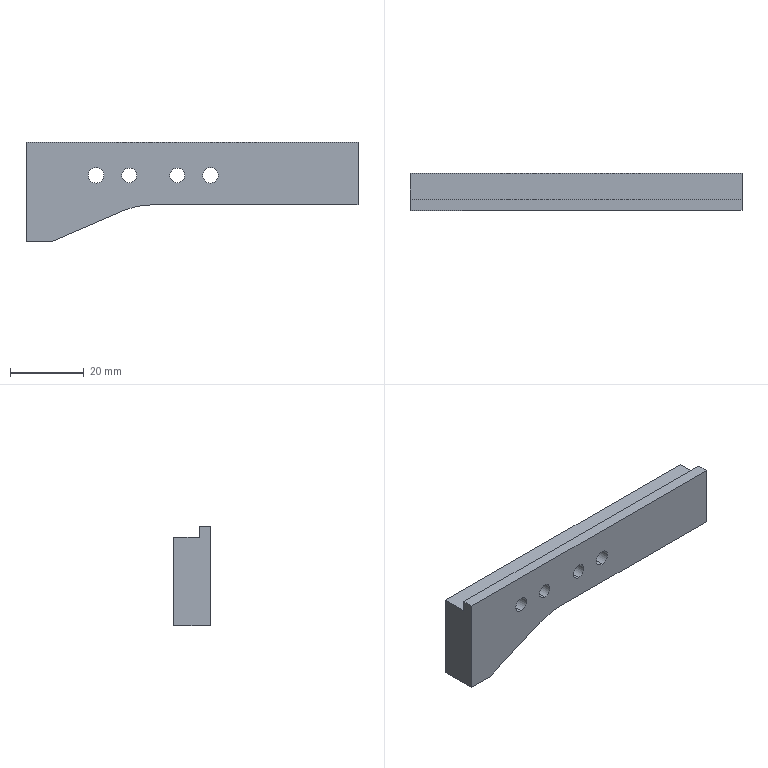Part | STEP file | PN_0060 | 1 solid | 19 faces | box 90 x 10 x 27 mm | volume 14739 mm3 | plane 10 | cylinder 9 | commonest cylinder face diameters 4 x4 4.2 x4 40 x1
STEP:
#1=CARTESIAN_POINT('',(0.,0.,0.));
#2=DIRECTION('',(0.,0.,1.));
#3=DIRECTION('',(1.,0.,0.));
#4=AXIS2_PLACEMENT_3D('',#1,#2,#3);
#5=CARTESIAN_POINT('',(-32.,0.,1.5));
#6=VERTEX_POINT('',#5);
#7=CARTESIAN_POINT('',(-32.,10.,1.5));
#8=VERTEX_POINT('',#7);
#9=CARTESIAN_POINT('',(-32.,10.,1.5));
#10=DIRECTION('',(0.,1.,0.));
#11=VECTOR('',#10,1.);
#12=LINE('',#9,#11);
#13=CARTESIAN_POINT('',(-32.,10.,-0.5));
#14=DIRECTION('',(0.,1.,0.));
#15=DIRECTION('',(0.,0.,1.));
#16=AXIS2_PLACEMENT_3D('',#13,#14,#15);
#17=CYLINDRICAL_SURFACE('',#16,2.);
#18=CARTESIAN_POINT('',(6.283,0.));
#19=DIRECTION('',(0.,1.));
#20=VECTOR('',#19,1.);
#21=LINE('',#18,#20);
#22=(GEOMETRIC_REPRESENTATION_CONTEXT(2)PARAMETRIC_REPRESENTATION_CONTEXT()REPRESENTATION_CONTEXT('',''));
#23=DEFINITIONAL_REPRESENTATION('',(#21),#22);
#24=PCURVE('',#17,#23);
#25=CARTESIAN_POINT('',(-32.,10.,-0.5));
#26=DIRECTION('',(0.,1.,0.));
#27=DIRECTION('',(0.,0.,1.));
#28=AXIS2_PLACEMENT_3D('',#25,#26,#27);
#29=CYLINDRICAL_SURFACE('',#28,2.);
#30=CARTESIAN_POINT('',(0.,0.));
#31=DIRECTION('',(0.,1.));
#32=VECTOR('',#31,1.);
#33=LINE('',#30,#32);
#34=(GEOMETRIC_REPRESENTATION_CONTEXT(2)PARAMETRIC_REPRESENTATION_CONTEXT()REPRESENTATION_CONTEXT('',''));
#35=DEFINITIONAL_REPRESENTATION('',(#33),#34);
#36=PCURVE('',#29,#35);
#37=SURFACE_CURVE('',#12,(#24,#36),.PCURVE_S1.);
#38=EDGE_CURVE('',#6,#8,#37,.T.);
#39=ORIENTED_EDGE('',*,*,#38,.T.);
#40=CARTESIAN_POINT('',(-32.,10.,-2.5));
#41=VERTEX_POINT('',#40);
#42=CARTESIAN_POINT('',(-32.,10.,-0.5));
#43=DIRECTION('',(0.,1.,0.));
#44=DIRECTION('',(0.,0.,1.));
#45=AXIS2_PLACEMENT_3D('',#42,#43,#44);
#46=CIRCLE('',#45,2.);
#47=CARTESIAN_POINT('',(0.,0.));
#48=DIRECTION('',(1.,0.));
#49=VECTOR('',#48,1.);
#50=LINE('',#47,#49);
#51=(GEOMETRIC_REPRESENTATION_CONTEXT(2)PARAMETRIC_REPRESENTATION_CONTEXT()REPRESENTATION_CONTEXT('',''));
#52=DEFINITIONAL_REPRESENTATION('',(#50),#51);
#53=PCURVE('',#17,#52);
#54=CARTESIAN_POINT('',(0.,10.,0.));
#55=DIRECTION('',(0.,1.,0.));
#56=DIRECTION('',(0.,0.,1.));
#57=AXIS2_PLACEMENT_3D('',#54,#55,#56);
#58=PLANE('',#57);
#59=CARTESIAN_POINT('',(-0.5,-32.));
#60=DIRECTION('',(1.,0.));
#61=AXIS2_PLACEMENT_2D('',#59,#60);
#62=CIRCLE('',#61,2.);
#63=(GEOMETRIC_REPRESENTATION_CONTEXT(2)PARAMETRIC_REPRESENTATION_CONTEXT()REPRESENTATION_CONTEXT('',''));
#64=DEFINITIONAL_REPRESENTATION('',(#62),#63);
#65=PCURVE('',#58,#64);
#66=SURFACE_CURVE('',#46,(#53,#65),.PCURVE_S1.);
#67=EDGE_CURVE('',#41,#8,#66,.T.);
#68=ORIENTED_EDGE('',*,*,#67,.F.);
#69=CARTESIAN_POINT('',(-32.,0.,-2.5));
#70=VERTEX_POINT('',#69);
#71=CARTESIAN_POINT('',(-32.,10.,-2.5));
#72=DIRECTION('',(0.,1.,0.));
#73=VECTOR('',#72,1.);
#74=LINE('',#71,#73);
#75=CARTESIAN_POINT('',(3.142,0.));
#76=DIRECTION('',(0.,1.));
#77=VECTOR('',#76,1.);
#78=LINE('',#75,#77);
#79=(GEOMETRIC_REPRESENTATION_CONTEXT(2)PARAMETRIC_REPRESENTATION_CONTEXT()REPRESENTATION_CONTEXT('',''));
#80=DEFINITIONAL_REPRESENTATION('',(#78),#79);
#81=PCURVE('',#17,#80);
#82=CARTESIAN_POINT('',(3.142,0.));
#83=DIRECTION('',(0.,1.));
#84=VECTOR('',#83,1.);
#85=LINE('',#82,#84);
#86=(GEOMETRIC_REPRESENTATION_CONTEXT(2)PARAMETRIC_REPRESENTATION_CONTEXT()REPRESENTATION_CONTEXT('',''));
#87=DEFINITIONAL_REPRESENTATION('',(#85),#86);
#88=PCURVE('',#29,#87);
#89=SURFACE_CURVE('',#74,(#81,#88),.PCURVE_S1.);
#90=EDGE_CURVE('',#70,#41,#89,.T.);
#91=ORIENTED_EDGE('',*,*,#90,.F.);
#92=CARTESIAN_POINT('',(-32.,0.,-0.5));
#93=DIRECTION('',(0.,1.,0.));
#94=DIRECTION('',(0.,0.,1.));
#95=AXIS2_PLACEMENT_3D('',#92,#93,#94);
#96=CIRCLE('',#95,2.);
#97=CARTESIAN_POINT('',(0.,-10.));
#98=DIRECTION('',(1.,0.));
#99=VECTOR('',#98,1.);
#100=LINE('',#97,#99);
#101=(GEOMETRIC_REPRESENTATION_CONTEXT(2)PARAMETRIC_REPRESENTATION_CONTEXT()REPRESENTATION_CONTEXT('',''));
#102=DEFINITIONAL_REPRESENTATION('',(#100),#101);
#103=PCURVE('',#17,#102);
#104=CARTESIAN_POINT('',(0.,0.,0.));
#105=DIRECTION('',(0.,1.,0.));
#106=DIRECTION('',(0.,0.,1.));
#107=AXIS2_PLACEMENT_3D('',#104,#105,#106);
#108=PLANE('',#107);
#109=CARTESIAN_POINT('',(-0.5,-32.));
#110=DIRECTION('',(1.,0.));
#111=AXIS2_PLACEMENT_2D('',#109,#110);
#112=CIRCLE('',#111,2.);
#113=(GEOMETRIC_REPRESENTATION_CONTEXT(2)PARAMETRIC_REPRESENTATION_CONTEXT()REPRESENTATION_CONTEXT('',''));
#114=DEFINITIONAL_REPRESENTATION('',(#112),#113);
#115=PCURVE('',#108,#114);
#116=SURFACE_CURVE('',#96,(#103,#115),.PCURVE_S1.);
#117=EDGE_CURVE('',#70,#6,#116,.T.);
#118=ORIENTED_EDGE('',*,*,#117,.T.);
#119=EDGE_LOOP('',(#39,#68,#91,#118));
#120=FACE_BOUND('',#119,.F.);
#121=ADVANCED_FACE('',(#120),#17,.F.);
#122=CARTESIAN_POINT('',(-19.,0.,1.5));
#123=VERTEX_POINT('',#122);
#124=CARTESIAN_POINT('',(-19.,10.,1.5));
#125=VERTEX_POINT('',#124);
#126=CARTESIAN_POINT('',(-19.,10.,1.5));
#127=DIRECTION('',(0.,1.,0.));
#128=VECTOR('',#127,1.);
#129=LINE('',#126,#128);
#130=CARTESIAN_POINT('',(-19.,10.,-0.5));
#131=DIRECTION('',(0.,1.,0.));
#132=DIRECTION('',(0.,0.,1.));
#133=AXIS2_PLACEMENT_3D('',#130,#131,#132);
#134=CYLINDRICAL_SURFACE('',#133,2.);
#135=CARTESIAN_POINT('',(6.283,0.));
#136=DIRECTION('',(0.,1.));
#137=VECTOR('',#136,1.);
#138=LINE('',#135,#137);
#139=(GEOMETRIC_REPRESENTATION_CONTEXT(2)PARAMETRIC_REPRESENTATION_CONTEXT()REPRESENTATION_CONTEXT('',''));
#140=DEFINITIONAL_REPRESENTATION('',(#138),#139);
#141=PCURVE('',#134,#140);
#142=CARTESIAN_POINT('',(-19.,10.,-0.5));
#143=DIRECTION('',(0.,1.,0.));
#144=DIRECTION('',(0.,0.,1.));
#145=AXIS2_PLACEMENT_3D('',#142,#143,#144);
#146=CYLINDRICAL_SURFACE('',#145,2.);
#147=CARTESIAN_POINT('',(0.,0.));
#148=DIRECTION('',(0.,1.));
#149=VECTOR('',#148,1.);
#150=LINE('',#147,#149);
#151=(GEOMETRIC_REPRESENTATION_CONTEXT(2)PARAMETRIC_REPRESENTATION_CONTEXT()REPRESENTATION_CONTEXT('',''));
#152=DEFINITIONAL_REPRESENTATION('',(#150),#151);
#153=PCURVE('',#146,#152);
#154=SURFACE_CURVE('',#129,(#141,#153),.PCURVE_S1.);
#155=EDGE_CURVE('',#123,#125,#154,.T.);
#156=ORIENTED_EDGE('',*,*,#155,.T.);
#157=CARTESIAN_POINT('',(-19.,10.,-2.5));
#158=VERTEX_POINT('',#157);
#159=CARTESIAN_POINT('',(-19.,10.,-0.5));
#160=DIRECTION('',(0.,1.,0.));
#161=DIRECTION('',(0.,0.,1.));
#162=AXIS2_PLACEMENT_3D('',#159,#160,#161);
#163=CIRCLE('',#162,2.);
#164=CARTESIAN_POINT('',(0.,0.));
#165=DIRECTION('',(1.,0.));
#166=VECTOR('',#165,1.);
#167=LINE('',#164,#166);
#168=(GEOMETRIC_REPRESENTATION_CONTEXT(2)PARAMETRIC_REPRESENTATION_CONTEXT()REPRESENTATION_CONTEXT('',''));
#169=DEFINITIONAL_REPRESENTATION('',(#167),#168);
#170=PCURVE('',#134,#169);
#171=CARTESIAN_POINT('',(-0.5,-19.));
#172=DIRECTION('',(1.,0.));
#173=AXIS2_PLACEMENT_2D('',#171,#172);
#174=CIRCLE('',#173,2.);
#175=(GEOMETRIC_REPRESENTATION_CONTEXT(2)PARAMETRIC_REPRESENTATION_CONTEXT()REPRESENTATION_CONTEXT('',''));
#176=DEFINITIONAL_REPRESENTATION('',(#174),#175);
#177=PCURVE('',#58,#176);
#178=SURFACE_CURVE('',#163,(#170,#177),.PCURVE_S1.);
#179=EDGE_CURVE('',#158,#125,#178,.T.);
#180=ORIENTED_EDGE('',*,*,#179,.F.);
#181=CARTESIAN_POINT('',(-19.,0.,-2.5));
#182=VERTEX_POINT('',#181);
#183=CARTESIAN_POINT('',(-19.,10.,-2.5));
#184=DIRECTION('',(0.,1.,0.));
#185=VECTOR('',#184,1.);
#186=LINE('',#183,#185);
#187=CARTESIAN_POINT('',(3.142,0.));
#188=DIRECTION('',(0.,1.));
#189=VECTOR('',#188,1.);
#190=LINE('',#187,#189);
#191=(GEOMETRIC_REPRESENTATION_CONTEXT(2)PARAMETRIC_REPRESENTATION_CONTEXT()REPRESENTATION_CONTEXT('',''));
#192=DEFINITIONAL_REPRESENTATION('',(#190),#191);
#193=PCURVE('',#134,#192);
#194=CARTESIAN_POINT('',(3.142,0.));
#195=DIRECTION('',(0.,1.));
#196=VECTOR('',#195,1.);
#197=LINE('',#194,#196);
#198=(GEOMETRIC_REPRESENTATION_CONTEXT(2)PARAMETRIC_REPRESENTATION_CONTEXT()REPRESENTATION_CONTEXT('',''));
#199=DEFINITIONAL_REPRESENTATION('',(#197),#198);
#200=PCURVE('',#146,#199);
#201=SURFACE_CURVE('',#186,(#193,#200),.PCURVE_S1.);
#202=EDGE_CURVE('',#182,#158,#201,.T.);
#203=ORIENTED_EDGE('',*,*,#202,.F.);
#204=CARTESIAN_POINT('',(-19.,0.,-0.5));
#205=DIRECTION('',(0.,1.,0.));
#206=DIRECTION('',(0.,0.,1.));
#207=AXIS2_PLACEMENT_3D('',#204,#205,#206);
#208=CIRCLE('',#207,2.);
#209=CARTESIAN_POINT('',(0.,-10.));
#210=DIRECTION('',(1.,0.));
#211=VECTOR('',#210,1.);
#212=LINE('',#209,#211);
#213=(GEOMETRIC_REPRESENTATION_CONTEXT(2)PARAMETRIC_REPRESENTATION_CONTEXT()REPRESENTATION_CONTEXT('',''));
#214=DEFINITIONAL_REPRESENTATION('',(#212),#213);
#215=PCURVE('',#134,#214);
#216=CARTESIAN_POINT('',(-0.5,-19.));
#217=DIRECTION('',(1.,0.));
#218=AXIS2_PLACEMENT_2D('',#216,#217);
#219=CIRCLE('',#218,2.);
#220=(GEOMETRIC_REPRESENTATION_CONTEXT(2)PARAMETRIC_REPRESENTATION_CONTEXT()REPRESENTATION_CONTEXT('',''));
#221=DEFINITIONAL_REPRESENTATION('',(#219),#220);
#222=PCURVE('',#108,#221);
#223=SURFACE_CURVE('',#208,(#215,#222),.PCURVE_S1.);
#224=EDGE_CURVE('',#182,#123,#223,.T.);
#225=ORIENTED_EDGE('',*,*,#224,.T.);
#226=EDGE_LOOP('',(#156,#180,#203,#225));
#227=FACE_BOUND('',#226,.F.);
#228=ADVANCED_FACE('',(#227),#134,.F.);
#229=CARTESIAN_POINT('',(-41.,0.,1.6));
#230=VERTEX_POINT('',#229);
#231=CARTESIAN_POINT('',(-41.,10.,1.6));
#232=VERTEX_POINT('',#231);
#233=CARTESIAN_POINT('',(-41.,10.,1.6));
#234=DIRECTION('',(0.,1.,0.));
#235=VECTOR('',#234,1.);
#236=LINE('',#233,#235);
#237=CARTESIAN_POINT('',(-41.,10.,-0.5));
#238=DIRECTION('',(0.,1.,0.));
#239=DIRECTION('',(0.,0.,1.));
#240=AXIS2_PLACEMENT_3D('',#237,#238,#239);
#241=CYLINDRICAL_SURFACE('',#240,2.1);
#242=CARTESIAN_POINT('',(6.283,0.));
#243=DIRECTION('',(0.,1.));
#244=VECTOR('',#243,1.);
#245=LINE('',#242,#244);
#246=(GEOMETRIC_REPRESENTATION_CONTEXT(2)PARAMETRIC_REPRESENTATION_CONTEXT()REPRESENTATION_CONTEXT('',''));
#247=DEFINITIONAL_REPRESENTATION('',(#245),#246);
#248=PCURVE('',#241,#247);
#249=CARTESIAN_POINT('',(-41.,10.,-0.5));
#250=DIRECTION('',(0.,1.,0.));
#251=DIRECTION('',(0.,0.,1.));
#252=AXIS2_PLACEMENT_3D('',#249,#250,#251);
#253=CYLINDRICAL_SURFACE('',#252,2.1);
#254=CARTESIAN_POINT('',(0.,0.));
#255=DIRECTION('',(0.,1.));
#256=VECTOR('',#255,1.);
#257=LINE('',#254,#256);
#258=(GEOMETRIC_REPRESENTATION_CONTEXT(2)PARAMETRIC_REPRESENTATION_CONTEXT()REPRESENTATION_CONTEXT('',''));
#259=DEFINITIONAL_REPRESENTATION('',(#257),#258);
#260=PCURVE('',#253,#259);
#261=SURFACE_CURVE('',#236,(#248,#260),.PCURVE_S1.);
#262=EDGE_CURVE('',#230,#232,#261,.T.);
#263=ORIENTED_EDGE('',*,*,#262,.T.);
#264=CARTESIAN_POINT('',(-41.,10.,-2.6));
#265=VERTEX_POINT('',#264);
#266=CARTESIAN_POINT('',(-41.,10.,-0.5));
#267=DIRECTION('',(0.,1.,0.));
#268=DIRECTION('',(0.,0.,1.));
#269=AXIS2_PLACEMENT_3D('',#266,#267,#268);
#270=CIRCLE('',#269,2.1);
#271=CARTESIAN_POINT('',(0.,0.));
#272=DIRECTION('',(1.,0.));
#273=VECTOR('',#272,1.);
#274=LINE('',#271,#273);
#275=(GEOMETRIC_REPRESENTATION_CONTEXT(2)PARAMETRIC_REPRESENTATION_CONTEXT()REPRESENTATION_CONTEXT('',''));
#276=DEFINITIONAL_REPRESENTATION('',(#274),#275);
#277=PCURVE('',#241,#276);
#278=CARTESIAN_POINT('',(-0.5,-41.));
#279=DIRECTION('',(1.,0.));
#280=AXIS2_PLACEMENT_2D('',#278,#279);
#281=CIRCLE('',#280,2.1);
#282=(GEOMETRIC_REPRESENTATION_CONTEXT(2)PARAMETRIC_REPRESENTATION_CONTEXT()REPRESENTATION_CONTEXT('',''));
#283=DEFINITIONAL_REPRESENTATION('',(#281),#282);
#284=PCURVE('',#58,#283);
#285=SURFACE_CURVE('',#270,(#277,#284),.PCURVE_S1.);
#286=EDGE_CURVE('',#265,#232,#285,.T.);
#287=ORIENTED_EDGE('',*,*,#286,.F.);
#288=CARTESIAN_POINT('',(-41.,0.,-2.6));
#289=VERTEX_POINT('',#288);
#290=CARTESIAN_POINT('',(-41.,10.,-2.6));
#291=DIRECTION('',(0.,1.,0.));
#292=VECTOR('',#291,1.);
#293=LINE('',#290,#292);
#294=CARTESIAN_POINT('',(3.142,0.));
#295=DIRECTION('',(0.,1.));
#296=VECTOR('',#295,1.);
#297=LINE('',#294,#296);
#298=(GEOMETRIC_REPRESENTATION_CONTEXT(2)PARAMETRIC_REPRESENTATION_CONTEXT()REPRESENTATION_CONTEXT('',''));
#299=DEFINITIONAL_REPRESENTATION('',(#297),#298);
#300=PCURVE('',#241,#299);
#301=CARTESIAN_POINT('',(3.142,0.));
#302=DIRECTION('',(0.,1.));
#303=VECTOR('',#302,1.);
#304=LINE('',#301,#303);
#305=(GEOMETRIC_REPRESENTATION_CONTEXT(2)PARAMETRIC_REPRESENTATION_CONTEXT()REPRESENTATION_CONTEXT('',''));
#306=DEFINITIONAL_REPRESENTATION('',(#304),#305);
#307=PCURVE('',#253,#306);
#308=SURFACE_CURVE('',#293,(#300,#307),.PCURVE_S1.);
#309=EDGE_CURVE('',#289,#265,#308,.T.);
#310=ORIENTED_EDGE('',*,*,#309,.F.);
#311=CARTESIAN_POINT('',(-41.,0.,-0.5));
#312=DIRECTION('',(0.,1.,0.));
#313=DIRECTION('',(0.,0.,1.));
#314=AXIS2_PLACEMENT_3D('',#311,#312,#313);
#315=CIRCLE('',#314,2.1);
#316=CARTESIAN_POINT('',(0.,-10.));
#317=DIRECTION('',(1.,0.));
#318=VECTOR('',#317,1.);
#319=LINE('',#316,#318);
#320=(GEOMETRIC_REPRESENTATION_CONTEXT(2)PARAMETRIC_REPRESENTATION_CONTEXT()REPRESENTATION_CONTEXT('',''));
#321=DEFINITIONAL_REPRESENTATION('',(#319),#320);
#322=PCURVE('',#241,#321);
#323=CARTESIAN_POINT('',(-0.5,-41.));
#324=DIRECTION('',(1.,0.));
#325=AXIS2_PLACEMENT_2D('',#323,#324);
#326=CIRCLE('',#325,2.1);
#327=(GEOMETRIC_REPRESENTATION_CONTEXT(2)PARAMETRIC_REPRESENTATION_CONTEXT()REPRESENTATION_CONTEXT('',''));
#328=DEFINITIONAL_REPRESENTATION('',(#326),#327);
#329=PCURVE('',#108,#328);
#330=SURFACE_CURVE('',#315,(#322,#329),.PCURVE_S1.);
#331=EDGE_CURVE('',#289,#230,#330,.T.);
#332=ORIENTED_EDGE('',*,*,#331,.T.);
#333=EDGE_LOOP('',(#263,#287,#310,#332));
#334=FACE_BOUND('',#333,.F.);
#335=ADVANCED_FACE('',(#334),#241,.F.);
#336=CARTESIAN_POINT('',(-10.,0.,1.6));
#337=VERTEX_POINT('',#336);
#338=CARTESIAN_POINT('',(-10.,10.,1.6));
#339=VERTEX_POINT('',#338);
#340=CARTESIAN_POINT('',(-10.,10.,1.6));
#341=DIRECTION('',(0.,1.,0.));
#342=VECTOR('',#341,1.);
#343=LINE('',#340,#342);
#344=CARTESIAN_POINT('',(-10.,10.,-0.5));
#345=DIRECTION('',(0.,1.,0.));
#346=DIRECTION('',(0.,0.,1.));
#347=AXIS2_PLACEMENT_3D('',#344,#345,#346);
#348=CYLINDRICAL_SURFACE('',#347,2.1);
#349=CARTESIAN_POINT('',(6.283,0.));
#350=DIRECTION('',(0.,1.));
#351=VECTOR('',#350,1.);
#352=LINE('',#349,#351);
#353=(GEOMETRIC_REPRESENTATION_CONTEXT(2)PARAMETRIC_REPRESENTATION_CONTEXT()REPRESENTATION_CONTEXT('',''));
#354=DEFINITIONAL_REPRESENTATION('',(#352),#353);
#355=PCURVE('',#348,#354);
#356=CARTESIAN_POINT('',(-10.,10.,-0.5));
#357=DIRECTION('',(0.,1.,0.));
#358=DIRECTION('',(0.,0.,1.));
#359=AXIS2_PLACEMENT_3D('',#356,#357,#358);
#360=CYLINDRICAL_SURFACE('',#359,2.1);
#361=CARTESIAN_POINT('',(0.,0.));
#362=DIRECTION('',(0.,1.));
#363=VECTOR('',#362,1.);
#364=LINE('',#361,#363);
#365=(GEOMETRIC_REPRESENTATION_CONTEXT(2)PARAMETRIC_REPRESENTATION_CONTEXT()REPRESENTATION_CONTEXT('',''));
#366=DEFINITIONAL_REPRESENTATION('',(#364),#365);
#367=PCURVE('',#360,#366);
#368=SURFACE_CURVE('',#343,(#355,#367),.PCURVE_S1.);
#369=EDGE_CURVE('',#337,#339,#368,.T.);
#370=ORIENTED_EDGE('',*,*,#369,.T.);
#371=CARTESIAN_POINT('',(-10.,10.,-2.6));
#372=VERTEX_POINT('',#371);
#373=CARTESIAN_POINT('',(-10.,10.,-0.5));
#374=DIRECTION('',(0.,1.,0.));
#375=DIRECTION('',(0.,0.,1.));
#376=AXIS2_PLACEMENT_3D('',#373,#374,#375);
#377=CIRCLE('',#376,2.1);
#378=CARTESIAN_POINT('',(0.,0.));
#379=DIRECTION('',(1.,0.));
#380=VECTOR('',#379,1.);
#381=LINE('',#378,#380);
#382=(GEOMETRIC_REPRESENTATION_CONTEXT(2)PARAMETRIC_REPRESENTATION_CONTEXT()REPRESENTATION_CONTEXT('',''));
#383=DEFINITIONAL_REPRESENTATION('',(#381),#382);
#384=PCURVE('',#348,#383);
#385=CARTESIAN_POINT('',(-0.5,-10.));
#386=DIRECTION('',(1.,0.));
#387=AXIS2_PLACEMENT_2D('',#385,#386);
#388=CIRCLE('',#387,2.1);
#389=(GEOMETRIC_REPRESENTATION_CONTEXT(2)PARAMETRIC_REPRESENTATION_CONTEXT()REPRESENTATION_CONTEXT('',''));
#390=DEFINITIONAL_REPRESENTATION('',(#388),#389);
#391=PCURVE('',#58,#390);
#392=SURFACE_CURVE('',#377,(#384,#391),.PCURVE_S1.);
#393=EDGE_CURVE('',#372,#339,#392,.T.);
#394=ORIENTED_EDGE('',*,*,#393,.F.);
#395=CARTESIAN_POINT('',(-10.,0.,-2.6));
#396=VERTEX_POINT('',#395);
#397=CARTESIAN_POINT('',(-10.,10.,-2.6));
#398=DIRECTION('',(0.,1.,0.));
#399=VECTOR('',#398,1.);
#400=LINE('',#397,#399);
#401=CARTESIAN_POINT('',(3.142,0.));
#402=DIRECTION('',(0.,1.));
#403=VECTOR('',#402,1.);
#404=LINE('',#401,#403);
#405=(GEOMETRIC_REPRESENTATION_CONTEXT(2)PARAMETRIC_REPRESENTATION_CONTEXT()REPRESENTATION_CONTEXT('',''));
#406=DEFINITIONAL_REPRESENTATION('',(#404),#405);
#407=PCURVE('',#348,#406);
#408=CARTESIAN_POINT('',(3.142,0.));
#409=DIRECTION('',(0.,1.));
#410=VECTOR('',#409,1.);
#411=LINE('',#408,#410);
#412=(GEOMETRIC_REPRESENTATION_CONTEXT(2)PARAMETRIC_REPRESENTATION_CONTEXT()REPRESENTATION_CONTEXT('',''));
#413=DEFINITIONAL_REPRESENTATION('',(#411),#412);
#414=PCURVE('',#360,#413);
#415=SURFACE_CURVE('',#400,(#407,#414),.PCURVE_S1.);
#416=EDGE_CURVE('',#396,#372,#415,.T.);
#417=ORIENTED_EDGE('',*,*,#416,.F.);
#418=CARTESIAN_POINT('',(-10.,0.,-0.5));
#419=DIRECTION('',(0.,1.,0.));
#420=DIRECTION('',(0.,0.,1.));
#421=AXIS2_PLACEMENT_3D('',#418,#419,#420);
#422=CIRCLE('',#421,2.1);
#423=CARTESIAN_POINT('',(0.,-10.));
#424=DIRECTION('',(1.,0.));
#425=VECTOR('',#424,1.);
#426=LINE('',#423,#425);
#427=(GEOMETRIC_REPRESENTATION_CONTEXT(2)PARAMETRIC_REPRESENTATION_CONTEXT()REPRESENTATION_CONTEXT('',''));
#428=DEFINITIONAL_REPRESENTATION('',(#426),#427);
#429=PCURVE('',#348,#428);
#430=CARTESIAN_POINT('',(-0.5,-10.));
#431=DIRECTION('',(1.,0.));
#432=AXIS2_PLACEMENT_2D('',#430,#431);
#433=CIRCLE('',#432,2.1);
#434=(GEOMETRIC_REPRESENTATION_CONTEXT(2)PARAMETRIC_REPRESENTATION_CONTEXT()REPRESENTATION_CONTEXT('',''));
#435=DEFINITIONAL_REPRESENTATION('',(#433),#434);
#436=PCURVE('',#108,#435);
#437=SURFACE_CURVE('',#422,(#429,#436),.PCURVE_S1.);
#438=EDGE_CURVE('',#396,#337,#437,.T.);
#439=ORIENTED_EDGE('',*,*,#438,.T.);
#440=EDGE_LOOP('',(#370,#394,#417,#439));
#441=FACE_BOUND('',#440,.F.);
#442=ADVANCED_FACE('',(#441),#348,.F.);
#443=CARTESIAN_POINT('',(30.,10.,5.5));
#444=VERTEX_POINT('',#443);
#445=CARTESIAN_POINT('',(30.,3.,5.5));
#446=VERTEX_POINT('',#445);
#447=CARTESIAN_POINT('',(30.,10.,5.5));
#448=DIRECTION('',(0.,-1.,0.));
#449=VECTOR('',#448,1.);
#450=LINE('',#447,#449);
#451=CARTESIAN_POINT('',(30.,10.,-8.5));
#452=DIRECTION('',(-1.,0.,0.));
#453=DIRECTION('',(0.,0.,1.));
#454=AXIS2_PLACEMENT_3D('',#451,#452,#453);
#455=PLANE('',#454);
#456=CARTESIAN_POINT('',(14.,0.));
#457=DIRECTION('',(0.,-1.));
#458=VECTOR('',#457,1.);
#459=LINE('',#456,#458);
#460=(GEOMETRIC_REPRESENTATION_CONTEXT(2)PARAMETRIC_REPRESENTATION_CONTEXT()REPRESENTATION_CONTEXT('',''));
#461=DEFINITIONAL_REPRESENTATION('',(#459),#460);
#462=PCURVE('',#455,#461);
#463=CARTESIAN_POINT('',(48.,3.,5.5));
#464=DIRECTION('',(0.,0.,-1.));
#465=DIRECTION('',(-1.,0.,0.));
#466=AXIS2_PLACEMENT_3D('',#463,#464,#465);
#467=PLANE('',#466);
#468=CARTESIAN_POINT('',(18.,7.));
#469=DIRECTION('',(0.,-1.));
#470=VECTOR('',#469,1.);
#471=LINE('',#468,#470);
#472=(GEOMETRIC_REPRESENTATION_CONTEXT(2)PARAMETRIC_REPRESENTATION_CONTEXT()REPRESENTATION_CONTEXT('',''));
#473=DEFINITIONAL_REPRESENTATION('',(#471),#472);
#474=PCURVE('',#467,#473);
#475=SURFACE_CURVE('',#450,(#462,#474),.PCURVE_S1.);
#476=EDGE_CURVE('',#444,#446,#475,.T.);
#477=ORIENTED_EDGE('',*,*,#476,.T.);
#478=CARTESIAN_POINT('',(30.,3.,8.5));
#479=VERTEX_POINT('',#478);
#480=CARTESIAN_POINT('',(30.,3.,-8.5));
#481=DIRECTION('',(0.,0.,1.));
#482=VECTOR('',#481,1.);
#483=LINE('',#480,#482);
#484=CARTESIAN_POINT('',(0.,-7.));
#485=DIRECTION('',(1.,0.));
#486=VECTOR('',#485,1.);
#487=LINE('',#484,#486);
#488=(GEOMETRIC_REPRESENTATION_CONTEXT(2)PARAMETRIC_REPRESENTATION_CONTEXT()REPRESENTATION_CONTEXT('',''));
#489=DEFINITIONAL_REPRESENTATION('',(#487),#488);
#490=PCURVE('',#455,#489);
#491=CARTESIAN_POINT('',(48.,3.,8.5));
#492=DIRECTION('',(0.,-1.,0.));
#493=DIRECTION('',(0.,0.,-1.));
#494=AXIS2_PLACEMENT_3D('',#491,#492,#493);
#495=PLANE('',#494);
#496=CARTESIAN_POINT('',(17.,-18.));
#497=DIRECTION('',(-1.,0.));
#498=VECTOR('',#497,1.);
#499=LINE('',#496,#498);
#500=(GEOMETRIC_REPRESENTATION_CONTEXT(2)PARAMETRIC_REPRESENTATION_CONTEXT()REPRESENTATION_CONTEXT('',''));
#501=DEFINITIONAL_REPRESENTATION('',(#499),#500);
#502=PCURVE('',#495,#501);
#503=SURFACE_CURVE('',#483,(#490,#502),.PCURVE_S1.);
#504=EDGE_CURVE('',#446,#479,#503,.T.);
#505=ORIENTED_EDGE('',*,*,#504,.T.);
#506=CARTESIAN_POINT('',(30.,0.,8.5));
#507=VERTEX_POINT('',#506);
#508=CARTESIAN_POINT('',(30.,10.,8.5));
#509=DIRECTION('',(0.,-1.,0.));
#510=VECTOR('',#509,1.);
#511=LINE('',#508,#510);
#512=CARTESIAN_POINT('',(17.,0.));
#513=DIRECTION('',(0.,-1.));
#514=VECTOR('',#513,1.);
#515=LINE('',#512,#514);
#516=(GEOMETRIC_REPRESENTATION_CONTEXT(2)PARAMETRIC_REPRESENTATION_CONTEXT()REPRESENTATION_CONTEXT('',''));
#517=DEFINITIONAL_REPRESENTATION('',(#515),#516);
#518=PCURVE('',#455,#517);
#519=CARTESIAN_POINT('',(-30.,10.,8.5));
#520=DIRECTION('',(0.,0.,-1.));
#521=DIRECTION('',(-1.,0.,0.));
#522=AXIS2_PLACEMENT_3D('',#519,#520,#521);
#523=PLANE('',#522);
#524=CARTESIAN_POINT('',(-60.,0.));
#525=DIRECTION('',(0.,-1.));
#526=VECTOR('',#525,1.);
#527=LINE('',#524,#526);
#528=(GEOMETRIC_REPRESENTATION_CONTEXT(2)PARAMETRIC_REPRESENTATION_CONTEXT()REPRESENTATION_CONTEXT('',''));
#529=DEFINITIONAL_REPRESENTATION('',(#527),#528);
#530=PCURVE('',#523,#529);
#531=SURFACE_CURVE('',#511,(#518,#530),.PCURVE_S1.);
#532=EDGE_CURVE('',#479,#507,#531,.T.);
#533=ORIENTED_EDGE('',*,*,#532,.T.);
#534=CARTESIAN_POINT('',(30.,0.,-8.5));
#535=VERTEX_POINT('',#534);
#536=CARTESIAN_POINT('',(30.,0.,-8.5));
#537=DIRECTION('',(0.,0.,-1.));
#538=VECTOR('',#537,1.);
#539=LINE('',#536,#538);
#540=CARTESIAN_POINT('',(0.,-10.));
#541=DIRECTION('',(-1.,0.));
#542=VECTOR('',#541,1.);
#543=LINE('',#540,#542);
#544=(GEOMETRIC_REPRESENTATION_CONTEXT(2)PARAMETRIC_REPRESENTATION_CONTEXT()REPRESENTATION_CONTEXT('',''));
#545=DEFINITIONAL_REPRESENTATION('',(#543),#544);
#546=PCURVE('',#455,#545);
#547=CARTESIAN_POINT('',(-8.5,30.));
#548=DIRECTION('',(-1.,0.));
#549=VECTOR('',#548,1.);
#550=LINE('',#547,#549);
#551=(GEOMETRIC_REPRESENTATION_CONTEXT(2)PARAMETRIC_REPRESENTATION_CONTEXT()REPRESENTATION_CONTEXT('',''));
#552=DEFINITIONAL_REPRESENTATION('',(#550),#551);
#553=PCURVE('',#108,#552);
#554=SURFACE_CURVE('',#539,(#546,#553),.PCURVE_S1.);
#555=EDGE_CURVE('',#507,#535,#554,.T.);
#556=ORIENTED_EDGE('',*,*,#555,.T.);
#557=CARTESIAN_POINT('',(30.,10.,-8.5));
#558=VERTEX_POINT('',#557);
#559=CARTESIAN_POINT('',(30.,10.,-8.5));
#560=DIRECTION('',(0.,-1.,0.));
#561=VECTOR('',#560,1.);
#562=LINE('',#559,#561);
#563=CARTESIAN_POINT('',(0.,0.));
#564=DIRECTION('',(0.,-1.));
#565=VECTOR('',#564,1.);
#566=LINE('',#563,#565);
#567=(GEOMETRIC_REPRESENTATION_CONTEXT(2)PARAMETRIC_REPRESENTATION_CONTEXT()REPRESENTATION_CONTEXT('',''));
#568=DEFINITIONAL_REPRESENTATION('',(#566),#567);
#569=PCURVE('',#455,#568);
#570=CARTESIAN_POINT('',(-30.,10.,-8.5));
#571=DIRECTION('',(0.,0.,1.));
#572=DIRECTION('',(1.,0.,0.));
#573=AXIS2_PLACEMENT_3D('',#570,#571,#572);
#574=PLANE('',#573);
#575=CARTESIAN_POINT('',(60.,0.));
#576=DIRECTION('',(0.,-1.));
#577=VECTOR('',#576,1.);
#578=LINE('',#575,#577);
#579=(GEOMETRIC_REPRESENTATION_CONTEXT(2)PARAMETRIC_REPRESENTATION_CONTEXT()REPRESENTATION_CONTEXT('',''));
#580=DEFINITIONAL_REPRESENTATION('',(#578),#579);
#581=PCURVE('',#574,#580);
#582=SURFACE_CURVE('',#562,(#569,#581),.PCURVE_S1.);
#583=EDGE_CURVE('',#558,#535,#582,.T.);
#584=ORIENTED_EDGE('',*,*,#583,.F.);
#585=CARTESIAN_POINT('',(30.,10.,-8.5));
#586=DIRECTION('',(0.,0.,-1.));
#587=VECTOR('',#586,1.);
#588=LINE('',#585,#587);
#589=CARTESIAN_POINT('',(0.,0.));
#590=DIRECTION('',(-1.,0.));
#591=VECTOR('',#590,1.);
#592=LINE('',#589,#591);
#593=(GEOMETRIC_REPRESENTATION_CONTEXT(2)PARAMETRIC_REPRESENTATION_CONTEXT()REPRESENTATION_CONTEXT('',''));
#594=DEFINITIONAL_REPRESENTATION('',(#592),#593);
#595=PCURVE('',#455,#594);
#596=CARTESIAN_POINT('',(-8.5,30.));
#597=DIRECTION('',(-1.,0.));
#598=VECTOR('',#597,1.);
#599=LINE('',#596,#598);
#600=(GEOMETRIC_REPRESENTATION_CONTEXT(2)PARAMETRIC_REPRESENTATION_CONTEXT()REPRESENTATION_CONTEXT('',''));
#601=DEFINITIONAL_REPRESENTATION('',(#599),#600);
#602=PCURVE('',#58,#601);
#603=SURFACE_CURVE('',#588,(#595,#602),.PCURVE_S1.);
#604=EDGE_CURVE('',#444,#558,#603,.T.);
#605=ORIENTED_EDGE('',*,*,#604,.F.);
#606=EDGE_LOOP('',(#477,#505,#533,#556,#584,#605));
#607=FACE_BOUND('',#606,.T.);
#608=ADVANCED_FACE('',(#607),#455,.F.);
#609=CARTESIAN_POINT('',(-25.853,0.,-8.5));
#610=VERTEX_POINT('',#609);
#611=CARTESIAN_POINT('',(-30.,0.,-8.5));
#612=DIRECTION('',(-1.,0.,0.));
#613=VECTOR('',#612,1.);
#614=LINE('',#611,#613);
#615=CARTESIAN_POINT('',(0.,-10.));
#616=DIRECTION('',(-1.,0.));
#617=VECTOR('',#616,1.);
#618=LINE('',#615,#617);
#619=(GEOMETRIC_REPRESENTATION_CONTEXT(2)PARAMETRIC_REPRESENTATION_CONTEXT()REPRESENTATION_CONTEXT('',''));
#620=DEFINITIONAL_REPRESENTATION('',(#618),#619);
#621=PCURVE('',#574,#620);
#622=CARTESIAN_POINT('',(-8.5,-30.));
#623=DIRECTION('',(0.,-1.));
#624=VECTOR('',#623,1.);
#625=LINE('',#622,#624);
#626=(GEOMETRIC_REPRESENTATION_CONTEXT(2)PARAMETRIC_REPRESENTATION_CONTEXT()REPRESENTATION_CONTEXT('',''));
#627=DEFINITIONAL_REPRESENTATION('',(#625),#626);
#628=PCURVE('',#108,#627);
#629=SURFACE_CURVE('',#614,(#621,#628),.PCURVE_S1.);
#630=EDGE_CURVE('',#535,#610,#629,.T.);
#631=ORIENTED_EDGE('',*,*,#630,.T.);
#632=CARTESIAN_POINT('',(-25.853,10.,-8.5));
#633=VERTEX_POINT('',#632);
#634=CARTESIAN_POINT('',(-25.853,10.,-8.5));
#635=DIRECTION('',(0.,1.,0.));
#636=VECTOR('',#635,1.);
#637=LINE('',#634,#636);
#638=CARTESIAN_POINT('',(4.147,0.));
#639=DIRECTION('',(0.,1.));
#640=VECTOR('',#639,1.);
#641=LINE('',#638,#640);
#642=(GEOMETRIC_REPRESENTATION_CONTEXT(2)PARAMETRIC_REPRESENTATION_CONTEXT()REPRESENTATION_CONTEXT('',''));
#643=DEFINITIONAL_REPRESENTATION('',(#641),#642);
#644=PCURVE('',#574,#643);
#645=CARTESIAN_POINT('',(-25.853,10.,-28.5));
#646=DIRECTION('',(0.,-1.,0.));
#647=DIRECTION('',(0.,0.,-1.));
#648=AXIS2_PLACEMENT_3D('',#645,#646,#647);
#649=CYLINDRICAL_SURFACE('',#648,20.);
#650=CARTESIAN_POINT('',(3.142,0.));
#651=DIRECTION('',(0.,-1.));
#652=VECTOR('',#651,1.);
#653=LINE('',#650,#652);
#654=(GEOMETRIC_REPRESENTATION_CONTEXT(2)PARAMETRIC_REPRESENTATION_CONTEXT()REPRESENTATION_CONTEXT('',''));
#655=DEFINITIONAL_REPRESENTATION('',(#653),#654);
#656=PCURVE('',#649,#655);
#657=SURFACE_CURVE('',#637,(#644,#656),.PCURVE_S1.);
#658=EDGE_CURVE('',#610,#633,#657,.T.);
#659=ORIENTED_EDGE('',*,*,#658,.T.);
#660=CARTESIAN_POINT('',(-30.,10.,-8.5));
#661=DIRECTION('',(-1.,0.,0.));
#662=VECTOR('',#661,1.);
#663=LINE('',#660,#662);
#664=CARTESIAN_POINT('',(0.,0.));
#665=DIRECTION('',(-1.,0.));
#666=VECTOR('',#665,1.);
#667=LINE('',#664,#666);
#668=(GEOMETRIC_REPRESENTATION_CONTEXT(2)PARAMETRIC_REPRESENTATION_CONTEXT()REPRESENTATION_CONTEXT('',''));
#669=DEFINITIONAL_REPRESENTATION('',(#667),#668);
#670=PCURVE('',#574,#669);
#671=CARTESIAN_POINT('',(-8.5,-30.));
#672=DIRECTION('',(0.,-1.));
#673=VECTOR('',#672,1.);
#674=LINE('',#671,#673);
#675=(GEOMETRIC_REPRESENTATION_CONTEXT(2)PARAMETRIC_REPRESENTATION_CONTEXT()REPRESENTATION_CONTEXT('',''));
#676=DEFINITIONAL_REPRESENTATION('',(#674),#675);
#677=PCURVE('',#58,#676);
#678=SURFACE_CURVE('',#663,(#670,#677),.PCURVE_S1.);
#679=EDGE_CURVE('',#558,#633,#678,.T.);
#680=ORIENTED_EDGE('',*,*,#679,.F.);
#681=ORIENTED_EDGE('',*,*,#583,.T.);
#682=EDGE_LOOP('',(#631,#659,#680,#681));
#683=FACE_BOUND('',#682,.T.);
#684=ADVANCED_FACE('',(#683),#574,.F.);
#685=ORIENTED_EDGE('',*,*,#532,.F.);
#686=CARTESIAN_POINT('',(-60.,3.,8.5));
#687=VERTEX_POINT('',#686);
#688=CARTESIAN_POINT('',(48.,3.,8.5));
#689=DIRECTION('',(-1.,0.,0.));
#690=VECTOR('',#689,1.);
#691=LINE('',#688,#690);
#692=CARTESIAN_POINT('',(-78.,-7.));
#693=DIRECTION('',(1.,0.));
#694=VECTOR('',#693,1.);
#695=LINE('',#692,#694);
#696=(GEOMETRIC_REPRESENTATION_CONTEXT(2)PARAMETRIC_REPRESENTATION_CONTEXT()REPRESENTATION_CONTEXT('',''));
#697=DEFINITIONAL_REPRESENTATION('',(#695),#696);
#698=PCURVE('',#523,#697);
#699=CARTESIAN_POINT('',(0.,0.));
#700=DIRECTION('',(0.,-1.));
#701=VECTOR('',#700,1.);
#702=LINE('',#699,#701);
#703=(GEOMETRIC_REPRESENTATION_CONTEXT(2)PARAMETRIC_REPRESENTATION_CONTEXT()REPRESENTATION_CONTEXT('',''));
#704=DEFINITIONAL_REPRESENTATION('',(#702),#703);
#705=PCURVE('',#495,#704);
#706=SURFACE_CURVE('',#691,(#698,#705),.PCURVE_S1.);
#707=EDGE_CURVE('',#479,#687,#706,.T.);
#708=ORIENTED_EDGE('',*,*,#707,.T.);
#709=CARTESIAN_POINT('',(-60.,0.,8.5));
#710=VERTEX_POINT('',#709);
#711=CARTESIAN_POINT('',(-60.,10.,8.5));
#712=DIRECTION('',(0.,-1.,0.));
#713=VECTOR('',#712,1.);
#714=LINE('',#711,#713);
#715=CARTESIAN_POINT('',(30.,0.));
#716=DIRECTION('',(0.,-1.));
#717=VECTOR('',#716,1.);
#718=LINE('',#715,#717);
#719=(GEOMETRIC_REPRESENTATION_CONTEXT(2)PARAMETRIC_REPRESENTATION_CONTEXT()REPRESENTATION_CONTEXT('',''));
#720=DEFINITIONAL_REPRESENTATION('',(#718),#719);
#721=PCURVE('',#523,#720);
#722=CARTESIAN_POINT('',(-60.,10.,8.5));
#723=DIRECTION('',(-1.,0.,0.));
#724=DIRECTION('',(0.,0.,1.));
#725=AXIS2_PLACEMENT_3D('',#722,#723,#724);
#726=PLANE('',#725);
#727=CARTESIAN_POINT('',(0.,0.));
#728=DIRECTION('',(0.,-1.));
#729=VECTOR('',#728,1.);
#730=LINE('',#727,#729);
#731=(GEOMETRIC_REPRESENTATION_CONTEXT(2)PARAMETRIC_REPRESENTATION_CONTEXT()REPRESENTATION_CONTEXT('',''));
#732=DEFINITIONAL_REPRESENTATION('',(#730),#731);
#733=PCURVE('',#726,#732);
#734=SURFACE_CURVE('',#714,(#721,#733),.PCURVE_S1.);
#735=EDGE_CURVE('',#687,#710,#734,.T.);
#736=ORIENTED_EDGE('',*,*,#735,.T.);
#737=CARTESIAN_POINT('',(-30.,0.,8.5));
#738=DIRECTION('',(1.,0.,0.));
#739=VECTOR('',#738,1.);
#740=LINE('',#737,#739);
#741=CARTESIAN_POINT('',(0.,-10.));
#742=DIRECTION('',(-1.,0.));
#743=VECTOR('',#742,1.);
#744=LINE('',#741,#743);
#745=(GEOMETRIC_REPRESENTATION_CONTEXT(2)PARAMETRIC_REPRESENTATION_CONTEXT()REPRESENTATION_CONTEXT('',''));
#746=DEFINITIONAL_REPRESENTATION('',(#744),#745);
#747=PCURVE('',#523,#746);
#748=CARTESIAN_POINT('',(8.5,-30.));
#749=DIRECTION('',(0.,1.));
#750=VECTOR('',#749,1.);
#751=LINE('',#748,#750);
#752=(GEOMETRIC_REPRESENTATION_CONTEXT(2)PARAMETRIC_REPRESENTATION_CONTEXT()REPRESENTATION_CONTEXT('',''));
#753=DEFINITIONAL_REPRESENTATION('',(#751),#752);
#754=PCURVE('',#108,#753);
#755=SURFACE_CURVE('',#740,(#747,#754),.PCURVE_S1.);
#756=EDGE_CURVE('',#710,#507,#755,.T.);
#757=ORIENTED_EDGE('',*,*,#756,.T.);
#758=EDGE_LOOP('',(#685,#708,#736,#757));
#759=FACE_BOUND('',#758,.T.);
#760=ADVANCED_FACE('',(#759),#523,.F.);
#761=CARTESIAN_POINT('',(-60.,10.,-18.5));
#762=VERTEX_POINT('',#761);
#763=CARTESIAN_POINT('',(-53.077,10.,-18.5));
#764=VERTEX_POINT('',#763);
#765=CARTESIAN_POINT('',(-60.,10.,-18.5));
#766=DIRECTION('',(1.,0.,0.));
#767=VECTOR('',#766,1.);
#768=LINE('',#765,#767);
#769=CARTESIAN_POINT('',(-18.5,-60.));
#770=DIRECTION('',(0.,1.));
#771=VECTOR('',#770,1.);
#772=LINE('',#769,#771);
#773=(GEOMETRIC_REPRESENTATION_CONTEXT(2)PARAMETRIC_REPRESENTATION_CONTEXT()REPRESENTATION_CONTEXT('',''));
#774=DEFINITIONAL_REPRESENTATION('',(#772),#773);
#775=PCURVE('',#58,#774);
#776=CARTESIAN_POINT('',(-60.,-12.,-18.5));
#777=DIRECTION('',(0.,0.,1.));
#778=DIRECTION('',(1.,0.,0.));
#779=AXIS2_PLACEMENT_3D('',#776,#777,#778);
#780=PLANE('',#779);
#781=CARTESIAN_POINT('',(0.,22.));
#782=DIRECTION('',(1.,0.));
#783=VECTOR('',#782,1.);
#784=LINE('',#781,#783);
#785=(GEOMETRIC_REPRESENTATION_CONTEXT(2)PARAMETRIC_REPRESENTATION_CONTEXT()REPRESENTATION_CONTEXT('',''));
#786=DEFINITIONAL_REPRESENTATION('',(#784),#785);
#787=PCURVE('',#780,#786);
#788=SURFACE_CURVE('',#768,(#775,#787),.PCURVE_S1.);
#789=EDGE_CURVE('',#762,#764,#788,.T.);
#790=ORIENTED_EDGE('',*,*,#789,.F.);
#791=CARTESIAN_POINT('',(-60.,10.,5.5));
#792=VERTEX_POINT('',#791);
#793=CARTESIAN_POINT('',(-60.,10.,8.5));
#794=DIRECTION('',(0.,0.,-1.));
#795=VECTOR('',#794,1.);
#796=LINE('',#793,#795);
#797=CARTESIAN_POINT('',(8.5,-60.));
#798=DIRECTION('',(-1.,0.));
#799=VECTOR('',#798,1.);
#800=LINE('',#797,#799);
#801=(GEOMETRIC_REPRESENTATION_CONTEXT(2)PARAMETRIC_REPRESENTATION_CONTEXT()REPRESENTATION_CONTEXT('',''));
#802=DEFINITIONAL_REPRESENTATION('',(#800),#801);
#803=PCURVE('',#58,#802);
#804=CARTESIAN_POINT('',(0.,0.));
#805=DIRECTION('',(-1.,0.));
#806=VECTOR('',#805,1.);
#807=LINE('',#804,#806);
#808=(GEOMETRIC_REPRESENTATION_CONTEXT(2)PARAMETRIC_REPRESENTATION_CONTEXT()REPRESENTATION_CONTEXT('',''));
#809=DEFINITIONAL_REPRESENTATION('',(#807),#808);
#810=PCURVE('',#726,#809);
#811=SURFACE_CURVE('',#796,(#803,#810),.PCURVE_S1.);
#812=EDGE_CURVE('',#792,#762,#811,.T.);
#813=ORIENTED_EDGE('',*,*,#812,.F.);
#814=CARTESIAN_POINT('',(48.,10.,5.5));
#815=DIRECTION('',(-1.,0.,0.));
#816=VECTOR('',#815,1.);
#817=LINE('',#814,#816);
#818=CARTESIAN_POINT('',(5.5,48.));
#819=DIRECTION('',(0.,-1.));
#820=VECTOR('',#819,1.);
#821=LINE('',#818,#820);
#822=(GEOMETRIC_REPRESENTATION_CONTEXT(2)PARAMETRIC_REPRESENTATION_CONTEXT()REPRESENTATION_CONTEXT('',''));
#823=DEFINITIONAL_REPRESENTATION('',(#821),#822);
#824=PCURVE('',#58,#823);
#825=CARTESIAN_POINT('',(0.,7.));
#826=DIRECTION('',(1.,0.));
#827=VECTOR('',#826,1.);
#828=LINE('',#825,#827);
#829=(GEOMETRIC_REPRESENTATION_CONTEXT(2)PARAMETRIC_REPRESENTATION_CONTEXT()REPRESENTATION_CONTEXT('',''));
#830=DEFINITIONAL_REPRESENTATION('',(#828),#829);
#831=PCURVE('',#467,#830);
#832=SURFACE_CURVE('',#817,(#824,#831),.PCURVE_S1.);
#833=EDGE_CURVE('',#444,#792,#832,.T.);
#834=ORIENTED_EDGE('',*,*,#833,.F.);
#835=ORIENTED_EDGE('',*,*,#604,.T.);
#836=ORIENTED_EDGE('',*,*,#679,.T.);
#837=CARTESIAN_POINT('',(-33.805,10.,-10.149));
#838=VERTEX_POINT('',#837);
#839=CARTESIAN_POINT('',(-25.853,10.,-28.5));
#840=DIRECTION('',(0.,-1.,0.));
#841=DIRECTION('',(0.,0.,1.));
#842=AXIS2_PLACEMENT_3D('',#839,#840,#841);
#843=CIRCLE('',#842,20.);
#844=CARTESIAN_POINT('',(-8.5,-25.853));
#845=CARTESIAN_POINT('',(-8.5,-60.494));
#846=CARTESIAN_POINT('',(-38.5,-43.173));
#847=CARTESIAN_POINT('',(-68.5,-25.853));
#848=CARTESIAN_POINT('',(-38.5,-8.532));
#849=CARTESIAN_POINT('',(-8.5,8.788));
#850=CARTESIAN_POINT('',(-8.5,-25.853));
#851=(BOUNDED_CURVE()B_SPLINE_CURVE(2,(#844,#845,#846,#847,#848,#849,#850),.UNSPECIFIED.,.T.,.F.)B_SPLINE_CURVE_WITH_KNOTS((1,2,2,2,2,1),(-2.094,0.,2.094,4.189,6.283,8.378),.UNSPECIFIED.)CURVE()GEOMETRIC_REPRESENTATION_ITEM()RATIONAL_B_SPLINE_CURVE((1.,0.5,1.,0.5,1.,0.5,1.))REPRESENTATION_ITEM(''));
#852=(GEOMETRIC_REPRESENTATION_CONTEXT(2)PARAMETRIC_REPRESENTATION_CONTEXT()REPRESENTATION_CONTEXT('',''));
#853=DEFINITIONAL_REPRESENTATION('',(#851),#852);
#854=PCURVE('',#58,#853);
#855=CARTESIAN_POINT('',(3.142,0.));
#856=DIRECTION('',(1.,0.));
#857=VECTOR('',#856,1.);
#858=LINE('',#855,#857);
#859=(GEOMETRIC_REPRESENTATION_CONTEXT(2)PARAMETRIC_REPRESENTATION_CONTEXT()REPRESENTATION_CONTEXT('',''));
#860=DEFINITIONAL_REPRESENTATION('',(#858),#859);
#861=PCURVE('',#649,#860);
#862=SURFACE_CURVE('',#843,(#854,#861),.PCURVE_S1.);
#863=EDGE_CURVE('',#633,#838,#862,.T.);
#864=ORIENTED_EDGE('',*,*,#863,.T.);
#865=CARTESIAN_POINT('',(-60.,10.,-21.5));
#866=DIRECTION('',(0.9176,0.,0.3976));
#867=VECTOR('',#866,1.);
#868=LINE('',#865,#867);
#869=CARTESIAN_POINT('',(-21.5,-60.));
#870=DIRECTION('',(0.3976,0.9176));
#871=VECTOR('',#870,1.);
#872=LINE('',#869,#871);
#873=(GEOMETRIC_REPRESENTATION_CONTEXT(2)PARAMETRIC_REPRESENTATION_CONTEXT()REPRESENTATION_CONTEXT('',''));
#874=DEFINITIONAL_REPRESENTATION('',(#872),#873);
#875=PCURVE('',#58,#874);
#876=CARTESIAN_POINT('',(-60.,10.,-21.5));
#877=DIRECTION('',(0.3976,0.,-0.9176));
#878=DIRECTION('',(-0.9176,0.,-0.3976));
#879=AXIS2_PLACEMENT_3D('',#876,#877,#878);
#880=PLANE('',#879);
#881=CARTESIAN_POINT('',(0.,0.));
#882=DIRECTION('',(-1.,0.));
#883=VECTOR('',#882,1.);
#884=LINE('',#881,#883);
#885=(GEOMETRIC_REPRESENTATION_CONTEXT(2)PARAMETRIC_REPRESENTATION_CONTEXT()REPRESENTATION_CONTEXT('',''));
#886=DEFINITIONAL_REPRESENTATION('',(#884),#885);
#887=PCURVE('',#880,#886);
#888=SURFACE_CURVE('',#868,(#875,#887),.PCURVE_S1.);
#889=EDGE_CURVE('',#764,#838,#888,.T.);
#890=ORIENTED_EDGE('',*,*,#889,.F.);
#891=EDGE_LOOP('',(#790,#813,#834,#835,#836,#864,#890));
#892=FACE_BOUND('',#891,.T.);
#893=CARTESIAN_POINT('',(-32.,10.,-0.5));
#894=DIRECTION('',(0.,1.,0.));
#895=DIRECTION('',(0.,0.,1.));
#896=AXIS2_PLACEMENT_3D('',#893,#894,#895);
#897=CIRCLE('',#896,2.);
#898=CARTESIAN_POINT('',(-0.5,-32.));
#899=DIRECTION('',(1.,0.));
#900=AXIS2_PLACEMENT_2D('',#898,#899);
#901=CIRCLE('',#900,2.);
#902=(GEOMETRIC_REPRESENTATION_CONTEXT(2)PARAMETRIC_REPRESENTATION_CONTEXT()REPRESENTATION_CONTEXT('',''));
#903=DEFINITIONAL_REPRESENTATION('',(#901),#902);
#904=PCURVE('',#58,#903);
#905=CARTESIAN_POINT('',(0.,0.));
#906=DIRECTION('',(1.,0.));
#907=VECTOR('',#906,1.);
#908=LINE('',#905,#907);
#909=(GEOMETRIC_REPRESENTATION_CONTEXT(2)PARAMETRIC_REPRESENTATION_CONTEXT()REPRESENTATION_CONTEXT('',''));
#910=DEFINITIONAL_REPRESENTATION('',(#908),#909);
#911=PCURVE('',#29,#910);
#912=SURFACE_CURVE('',#897,(#904,#911),.PCURVE_S1.);
#913=EDGE_CURVE('',#8,#41,#912,.T.);
#914=ORIENTED_EDGE('',*,*,#913,.F.);
#915=ORIENTED_EDGE('',*,*,#67,.F.);
#916=EDGE_LOOP('',(#914,#915));
#917=FACE_BOUND('',#916,.T.);
#918=CARTESIAN_POINT('',(-19.,10.,-0.5));
#919=DIRECTION('',(0.,1.,0.));
#920=DIRECTION('',(0.,0.,1.));
#921=AXIS2_PLACEMENT_3D('',#918,#919,#920);
#922=CIRCLE('',#921,2.);
#923=CARTESIAN_POINT('',(-0.5,-19.));
#924=DIRECTION('',(1.,0.));
#925=AXIS2_PLACEMENT_2D('',#923,#924);
#926=CIRCLE('',#925,2.);
#927=(GEOMETRIC_REPRESENTATION_CONTEXT(2)PARAMETRIC_REPRESENTATION_CONTEXT()REPRESENTATION_CONTEXT('',''));
#928=DEFINITIONAL_REPRESENTATION('',(#926),#927);
#929=PCURVE('',#58,#928);
#930=CARTESIAN_POINT('',(0.,0.));
#931=DIRECTION('',(1.,0.));
#932=VECTOR('',#931,1.);
#933=LINE('',#930,#932);
#934=(GEOMETRIC_REPRESENTATION_CONTEXT(2)PARAMETRIC_REPRESENTATION_CONTEXT()REPRESENTATION_CONTEXT('',''));
#935=DEFINITIONAL_REPRESENTATION('',(#933),#934);
#936=PCURVE('',#146,#935);
#937=SURFACE_CURVE('',#922,(#929,#936),.PCURVE_S1.);
#938=EDGE_CURVE('',#125,#158,#937,.T.);
#939=ORIENTED_EDGE('',*,*,#938,.F.);
#940=ORIENTED_EDGE('',*,*,#179,.F.);
#941=EDGE_LOOP('',(#939,#940));
#942=FACE_BOUND('',#941,.T.);
#943=CARTESIAN_POINT('',(-41.,10.,-0.5));
#944=DIRECTION('',(0.,1.,0.));
#945=DIRECTION('',(0.,0.,1.));
#946=AXIS2_PLACEMENT_3D('',#943,#944,#945);
#947=CIRCLE('',#946,2.1);
#948=CARTESIAN_POINT('',(-0.5,-41.));
#949=DIRECTION('',(1.,0.));
#950=AXIS2_PLACEMENT_2D('',#948,#949);
#951=CIRCLE('',#950,2.1);
#952=(GEOMETRIC_REPRESENTATION_CONTEXT(2)PARAMETRIC_REPRESENTATION_CONTEXT()REPRESENTATION_CONTEXT('',''));
#953=DEFINITIONAL_REPRESENTATION('',(#951),#952);
#954=PCURVE('',#58,#953);
#955=CARTESIAN_POINT('',(0.,0.));
#956=DIRECTION('',(1.,0.));
#957=VECTOR('',#956,1.);
#958=LINE('',#955,#957);
#959=(GEOMETRIC_REPRESENTATION_CONTEXT(2)PARAMETRIC_REPRESENTATION_CONTEXT()REPRESENTATION_CONTEXT('',''));
#960=DEFINITIONAL_REPRESENTATION('',(#958),#959);
#961=PCURVE('',#253,#960);
#962=SURFACE_CURVE('',#947,(#954,#961),.PCURVE_S1.);
#963=EDGE_CURVE('',#232,#265,#962,.T.);
#964=ORIENTED_EDGE('',*,*,#963,.F.);
#965=ORIENTED_EDGE('',*,*,#286,.F.);
#966=EDGE_LOOP('',(#964,#965));
#967=FACE_BOUND('',#966,.T.);
#968=CARTESIAN_POINT('',(-10.,10.,-0.5));
#969=DIRECTION('',(0.,1.,0.));
#970=DIRECTION('',(0.,0.,1.));
#971=AXIS2_PLACEMENT_3D('',#968,#969,#970);
#972=CIRCLE('',#971,2.1);
#973=CARTESIAN_POINT('',(-0.5,-10.));
#974=DIRECTION('',(1.,0.));
#975=AXIS2_PLACEMENT_2D('',#973,#974);
#976=CIRCLE('',#975,2.1);
#977=(GEOMETRIC_REPRESENTATION_CONTEXT(2)PARAMETRIC_REPRESENTATION_CONTEXT()REPRESENTATION_CONTEXT('',''));
#978=DEFINITIONAL_REPRESENTATION('',(#976),#977);
#979=PCURVE('',#58,#978);
#980=CARTESIAN_POINT('',(0.,0.));
#981=DIRECTION('',(1.,0.));
#982=VECTOR('',#981,1.);
#983=LINE('',#980,#982);
#984=(GEOMETRIC_REPRESENTATION_CONTEXT(2)PARAMETRIC_REPRESENTATION_CONTEXT()REPRESENTATION_CONTEXT('',''));
#985=DEFINITIONAL_REPRESENTATION('',(#983),#984);
#986=PCURVE('',#360,#985);
#987=SURFACE_CURVE('',#972,(#979,#986),.PCURVE_S1.);
#988=EDGE_CURVE('',#339,#372,#987,.T.);
#989=ORIENTED_EDGE('',*,*,#988,.F.);
#990=ORIENTED_EDGE('',*,*,#393,.F.);
#991=EDGE_LOOP('',(#989,#990));
#992=FACE_BOUND('',#991,.T.);
#993=ADVANCED_FACE('',(#892,#917,#942,#967,#992),#58,.T.);
#994=CARTESIAN_POINT('',(-32.,0.,-0.5));
#995=DIRECTION('',(0.,1.,0.));
#996=DIRECTION('',(0.,0.,1.));
#997=AXIS2_PLACEMENT_3D('',#994,#995,#996);
#998=CIRCLE('',#997,2.);
#999=CARTESIAN_POINT('',(-0.5,-32.));
#1000=DIRECTION('',(1.,0.));
#1001=AXIS2_PLACEMENT_2D('',#999,#1000);
#1002=CIRCLE('',#1001,2.);
#1003=(GEOMETRIC_REPRESENTATION_CONTEXT(2)PARAMETRIC_REPRESENTATION_CONTEXT()REPRESENTATION_CONTEXT('',''));
#1004=DEFINITIONAL_REPRESENTATION('',(#1002),#1003);
#1005=PCURVE('',#108,#1004);
#1006=CARTESIAN_POINT('',(0.,-10.));
#1007=DIRECTION('',(1.,0.));
#1008=VECTOR('',#1007,1.);
#1009=LINE('',#1006,#1008);
#1010=(GEOMETRIC_REPRESENTATION_CONTEXT(2)PARAMETRIC_REPRESENTATION_CONTEXT()REPRESENTATION_CONTEXT('',''));
#1011=DEFINITIONAL_REPRESENTATION('',(#1009),#1010);
#1012=PCURVE('',#29,#1011);
#1013=SURFACE_CURVE('',#998,(#1005,#1012),.PCURVE_S1.);
#1014=EDGE_CURVE('',#6,#70,#1013,.T.);
#1015=ORIENTED_EDGE('',*,*,#1014,.T.);
#1016=ORIENTED_EDGE('',*,*,#117,.T.);
#1017=EDGE_LOOP('',(#1015,#1016));
#1018=FACE_BOUND('',#1017,.T.);
#1019=CARTESIAN_POINT('',(-19.,0.,-0.5));
#1020=DIRECTION('',(0.,1.,0.));
#1021=DIRECTION('',(0.,0.,1.));
#1022=AXIS2_PLACEMENT_3D('',#1019,#1020,#1021);
#1023=CIRCLE('',#1022,2.);
#1024=CARTESIAN_POINT('',(-0.5,-19.));
#1025=DIRECTION('',(1.,0.));
#1026=AXIS2_PLACEMENT_2D('',#1024,#1025);
#1027=CIRCLE('',#1026,2.);
#1028=(GEOMETRIC_REPRESENTATION_CONTEXT(2)PARAMETRIC_REPRESENTATION_CONTEXT()REPRESENTATION_CONTEXT('',''));
#1029=DEFINITIONAL_REPRESENTATION('',(#1027),#1028);
#1030=PCURVE('',#108,#1029);
#1031=CARTESIAN_POINT('',(0.,-10.));
#1032=DIRECTION('',(1.,0.));
#1033=VECTOR('',#1032,1.);
#1034=LINE('',#1031,#1033);
#1035=(GEOMETRIC_REPRESENTATION_CONTEXT(2)PARAMETRIC_REPRESENTATION_CONTEXT()REPRESENTATION_CONTEXT('',''));
#1036=DEFINITIONAL_REPRESENTATION('',(#1034),#1035);
#1037=PCURVE('',#146,#1036);
#1038=SURFACE_CURVE('',#1023,(#1030,#1037),.PCURVE_S1.);
#1039=EDGE_CURVE('',#123,#182,#1038,.T.);
#1040=ORIENTED_EDGE('',*,*,#1039,.T.);
#1041=ORIENTED_EDGE('',*,*,#224,.T.);
#1042=EDGE_LOOP('',(#1040,#1041));
#1043=FACE_BOUND('',#1042,.T.);
#1044=CARTESIAN_POINT('',(-41.,0.,-0.5));
#1045=DIRECTION('',(0.,1.,0.));
#1046=DIRECTION('',(0.,0.,1.));
#1047=AXIS2_PLACEMENT_3D('',#1044,#1045,#1046);
#1048=CIRCLE('',#1047,2.1);
#1049=CARTESIAN_POINT('',(-0.5,-41.));
#1050=DIRECTION('',(1.,0.));
#1051=AXIS2_PLACEMENT_2D('',#1049,#1050);
#1052=CIRCLE('',#1051,2.1);
#1053=(GEOMETRIC_REPRESENTATION_CONTEXT(2)PARAMETRIC_REPRESENTATION_CONTEXT()REPRESENTATION_CONTEXT('',''));
#1054=DEFINITIONAL_REPRESENTATION('',(#1052),#1053);
#1055=PCURVE('',#108,#1054);
#1056=CARTESIAN_POINT('',(0.,-10.));
#1057=DIRECTION('',(1.,0.));
#1058=VECTOR('',#1057,1.);
#1059=LINE('',#1056,#1058);
#1060=(GEOMETRIC_REPRESENTATION_CONTEXT(2)PARAMETRIC_REPRESENTATION_CONTEXT()REPRESENTATION_CONTEXT('',''));
#1061=DEFINITIONAL_REPRESENTATION('',(#1059),#1060);
#1062=PCURVE('',#253,#1061);
#1063=SURFACE_CURVE('',#1048,(#1055,#1062),.PCURVE_S1.);
#1064=EDGE_CURVE('',#230,#289,#1063,.T.);
#1065=ORIENTED_EDGE('',*,*,#1064,.T.);
#1066=ORIENTED_EDGE('',*,*,#331,.T.);
#1067=EDGE_LOOP('',(#1065,#1066));
#1068=FACE_BOUND('',#1067,.T.);
#1069=CARTESIAN_POINT('',(-10.,0.,-0.5));
#1070=DIRECTION('',(0.,1.,0.));
#1071=DIRECTION('',(0.,0.,1.));
#1072=AXIS2_PLACEMENT_3D('',#1069,#1070,#1071);
#1073=CIRCLE('',#1072,2.1);
#1074=CARTESIAN_POINT('',(-0.5,-10.));
#1075=DIRECTION('',(1.,0.));
#1076=AXIS2_PLACEMENT_2D('',#1074,#1075);
#1077=CIRCLE('',#1076,2.1);
#1078=(GEOMETRIC_REPRESENTATION_CONTEXT(2)PARAMETRIC_REPRESENTATION_CONTEXT()REPRESENTATION_CONTEXT('',''));
#1079=DEFINITIONAL_REPRESENTATION('',(#1077),#1078);
#1080=PCURVE('',#108,#1079);
#1081=CARTESIAN_POINT('',(0.,-10.));
#1082=DIRECTION('',(1.,0.));
#1083=VECTOR('',#1082,1.);
#1084=LINE('',#1081,#1083);
#1085=(GEOMETRIC_REPRESENTATION_CONTEXT(2)PARAMETRIC_REPRESENTATION_CONTEXT()REPRESENTATION_CONTEXT('',''));
#1086=DEFINITIONAL_REPRESENTATION('',(#1084),#1085);
#1087=PCURVE('',#360,#1086);
#1088=SURFACE_CURVE('',#1073,(#1080,#1087),.PCURVE_S1.);
#1089=EDGE_CURVE('',#337,#396,#1088,.T.);
#1090=ORIENTED_EDGE('',*,*,#1089,.T.);
#1091=ORIENTED_EDGE('',*,*,#438,.T.);
#1092=EDGE_LOOP('',(#1090,#1091));
#1093=FACE_BOUND('',#1092,.T.);
#1094=CARTESIAN_POINT('',(-60.,0.,-18.5));
#1095=VERTEX_POINT('',#1094);
#1096=CARTESIAN_POINT('',(-60.,0.,8.5));
#1097=DIRECTION('',(0.,0.,-1.));
#1098=VECTOR('',#1097,1.);
#1099=LINE('',#1096,#1098);
#1100=CARTESIAN_POINT('',(8.5,-60.));
#1101=DIRECTION('',(-1.,0.));
#1102=VECTOR('',#1101,1.);
#1103=LINE('',#1100,#1102);
#1104=(GEOMETRIC_REPRESENTATION_CONTEXT(2)PARAMETRIC_REPRESENTATION_CONTEXT()REPRESENTATION_CONTEXT('',''));
#1105=DEFINITIONAL_REPRESENTATION('',(#1103),#1104);
#1106=PCURVE('',#108,#1105);
#1107=CARTESIAN_POINT('',(0.,-10.));
#1108=DIRECTION('',(-1.,0.));
#1109=VECTOR('',#1108,1.);
#1110=LINE('',#1107,#1109);
#1111=(GEOMETRIC_REPRESENTATION_CONTEXT(2)PARAMETRIC_REPRESENTATION_CONTEXT()REPRESENTATION_CONTEXT('',''));
#1112=DEFINITIONAL_REPRESENTATION('',(#1110),#1111);
#1113=PCURVE('',#726,#1112);
#1114=SURFACE_CURVE('',#1099,(#1106,#1113),.PCURVE_S1.);
#1115=EDGE_CURVE('',#710,#1095,#1114,.T.);
#1116=ORIENTED_EDGE('',*,*,#1115,.T.);
#1117=CARTESIAN_POINT('',(-53.077,0.,-18.5));
#1118=VERTEX_POINT('',#1117);
#1119=CARTESIAN_POINT('',(0.,0.,-18.5));
#1120=DIRECTION('',(1.,0.,0.));
#1121=VECTOR('',#1120,1.);
#1122=LINE('',#1119,#1121);
#1123=CARTESIAN_POINT('',(-18.5,0.));
#1124=DIRECTION('',(0.,1.));
#1125=VECTOR('',#1124,1.);
#1126=LINE('',#1123,#1125);
#1127=(GEOMETRIC_REPRESENTATION_CONTEXT(2)PARAMETRIC_REPRESENTATION_CONTEXT()REPRESENTATION_CONTEXT('',''));
#1128=DEFINITIONAL_REPRESENTATION('',(#1126),#1127);
#1129=PCURVE('',#108,#1128);
#1130=CARTESIAN_POINT('',(60.,12.));
#1131=DIRECTION('',(1.,0.));
#1132=VECTOR('',#1131,1.);
#1133=LINE('',#1130,#1132);
#1134=(GEOMETRIC_REPRESENTATION_CONTEXT(2)PARAMETRIC_REPRESENTATION_CONTEXT()REPRESENTATION_CONTEXT('',''));
#1135=DEFINITIONAL_REPRESENTATION('',(#1133),#1134);
#1136=PCURVE('',#780,#1135);
#1137=SURFACE_CURVE('',#1122,(#1129,#1136),.PCURVE_S1.);
#1138=EDGE_CURVE('',#1095,#1118,#1137,.T.);
#1139=ORIENTED_EDGE('',*,*,#1138,.T.);
#1140=CARTESIAN_POINT('',(-33.805,0.,-10.149));
#1141=VERTEX_POINT('',#1140);
#1142=CARTESIAN_POINT('',(-60.,0.,-21.5));
#1143=DIRECTION('',(0.9176,0.,0.3976));
#1144=VECTOR('',#1143,1.);
#1145=LINE('',#1142,#1144);
#1146=CARTESIAN_POINT('',(-21.5,-60.));
#1147=DIRECTION('',(0.3976,0.9176));
#1148=VECTOR('',#1147,1.);
#1149=LINE('',#1146,#1148);
#1150=(GEOMETRIC_REPRESENTATION_CONTEXT(2)PARAMETRIC_REPRESENTATION_CONTEXT()REPRESENTATION_CONTEXT('',''));
#1151=DEFINITIONAL_REPRESENTATION('',(#1149),#1150);
#1152=PCURVE('',#108,#1151);
#1153=CARTESIAN_POINT('',(0.,-10.));
#1154=DIRECTION('',(-1.,0.));
#1155=VECTOR('',#1154,1.);
#1156=LINE('',#1153,#1155);
#1157=(GEOMETRIC_REPRESENTATION_CONTEXT(2)PARAMETRIC_REPRESENTATION_CONTEXT()REPRESENTATION_CONTEXT('',''));
#1158=DEFINITIONAL_REPRESENTATION('',(#1156),#1157);
#1159=PCURVE('',#880,#1158);
#1160=SURFACE_CURVE('',#1145,(#1152,#1159),.PCURVE_S1.);
#1161=EDGE_CURVE('',#1118,#1141,#1160,.T.);
#1162=ORIENTED_EDGE('',*,*,#1161,.T.);
#1163=CARTESIAN_POINT('',(-25.853,0.,-28.5));
#1164=DIRECTION('',(0.,1.,0.));
#1165=DIRECTION('',(0.,0.,1.));
#1166=AXIS2_PLACEMENT_3D('',#1163,#1164,#1165);
#1167=CIRCLE('',#1166,20.);
#1168=CARTESIAN_POINT('',(-28.5,-25.853));
#1169=DIRECTION('',(1.,0.));
#1170=AXIS2_PLACEMENT_2D('',#1168,#1169);
#1171=CIRCLE('',#1170,20.);
#1172=(GEOMETRIC_REPRESENTATION_CONTEXT(2)PARAMETRIC_REPRESENTATION_CONTEXT()REPRESENTATION_CONTEXT('',''));
#1173=DEFINITIONAL_REPRESENTATION('',(#1171),#1172);
#1174=PCURVE('',#108,#1173);
#1175=CARTESIAN_POINT('',(9.425,10.));
#1176=DIRECTION('',(-1.,0.));
#1177=VECTOR('',#1176,1.);
#1178=LINE('',#1175,#1177);
#1179=(GEOMETRIC_REPRESENTATION_CONTEXT(2)PARAMETRIC_REPRESENTATION_CONTEXT()REPRESENTATION_CONTEXT('',''));
#1180=DEFINITIONAL_REPRESENTATION('',(#1178),#1179);
#1181=PCURVE('',#649,#1180);
#1182=SURFACE_CURVE('',#1167,(#1174,#1181),.PCURVE_S1.);
#1183=EDGE_CURVE('',#1141,#610,#1182,.T.);
#1184=ORIENTED_EDGE('',*,*,#1183,.T.);
#1185=ORIENTED_EDGE('',*,*,#630,.F.);
#1186=ORIENTED_EDGE('',*,*,#555,.F.);
#1187=ORIENTED_EDGE('',*,*,#756,.F.);
#1188=EDGE_LOOP('',(#1116,#1139,#1162,#1184,#1185,#1186,#1187));
#1189=FACE_BOUND('',#1188,.T.);
#1190=ADVANCED_FACE('',(#1018,#1043,#1068,#1093,#1189),#108,.F.);
#1191=CARTESIAN_POINT('',(-53.077,10.,-18.5));
#1192=DIRECTION('',(0.,-1.,0.));
#1193=VECTOR('',#1192,1.);
#1194=LINE('',#1191,#1193);
#1195=CARTESIAN_POINT('',(-7.545,0.));
#1196=DIRECTION('',(0.,-1.));
#1197=VECTOR('',#1196,1.);
#1198=LINE('',#1195,#1197);
#1199=(GEOMETRIC_REPRESENTATION_CONTEXT(2)PARAMETRIC_REPRESENTATION_CONTEXT()REPRESENTATION_CONTEXT('',''));
#1200=DEFINITIONAL_REPRESENTATION('',(#1198),#1199);
#1201=PCURVE('',#880,#1200);
#1202=CARTESIAN_POINT('',(6.923,22.));
#1203=DIRECTION('',(0.,-1.));
#1204=VECTOR('',#1203,1.);
#1205=LINE('',#1202,#1204);
#1206=(GEOMETRIC_REPRESENTATION_CONTEXT(2)PARAMETRIC_REPRESENTATION_CONTEXT()REPRESENTATION_CONTEXT('',''));
#1207=DEFINITIONAL_REPRESENTATION('',(#1205),#1206);
#1208=PCURVE('',#780,#1207);
#1209=SURFACE_CURVE('',#1194,(#1201,#1208),.PCURVE_S1.);
#1210=EDGE_CURVE('',#764,#1118,#1209,.T.);
#1211=ORIENTED_EDGE('',*,*,#1210,.F.);
#1212=ORIENTED_EDGE('',*,*,#889,.T.);
#1213=CARTESIAN_POINT('',(-33.805,10.,-10.149));
#1214=DIRECTION('',(0.,-1.,0.));
#1215=VECTOR('',#1214,1.);
#1216=LINE('',#1213,#1215);
#1217=CARTESIAN_POINT('',(-28.549,0.));
#1218=DIRECTION('',(0.,-1.));
#1219=VECTOR('',#1218,1.);
#1220=LINE('',#1217,#1219);
#1221=(GEOMETRIC_REPRESENTATION_CONTEXT(2)PARAMETRIC_REPRESENTATION_CONTEXT()REPRESENTATION_CONTEXT('',''));
#1222=DEFINITIONAL_REPRESENTATION('',(#1220),#1221);
#1223=PCURVE('',#880,#1222);
#1224=CARTESIAN_POINT('',(3.551,0.));
#1225=DIRECTION('',(0.,1.));
#1226=VECTOR('',#1225,1.);
#1227=LINE('',#1224,#1226);
#1228=(GEOMETRIC_REPRESENTATION_CONTEXT(2)PARAMETRIC_REPRESENTATION_CONTEXT()REPRESENTATION_CONTEXT('',''));
#1229=DEFINITIONAL_REPRESENTATION('',(#1227),#1228);
#1230=PCURVE('',#649,#1229);
#1231=SURFACE_CURVE('',#1216,(#1223,#1230),.PCURVE_S1.);
#1232=EDGE_CURVE('',#838,#1141,#1231,.T.);
#1233=ORIENTED_EDGE('',*,*,#1232,.T.);
#1234=ORIENTED_EDGE('',*,*,#1161,.F.);
#1235=EDGE_LOOP('',(#1211,#1212,#1233,#1234));
#1236=FACE_BOUND('',#1235,.T.);
#1237=ADVANCED_FACE('',(#1236),#880,.T.);
#1238=CARTESIAN_POINT('',(-60.,10.,-18.5));
#1239=DIRECTION('',(0.,1.,0.));
#1240=VECTOR('',#1239,1.);
#1241=LINE('',#1238,#1240);
#1242=CARTESIAN_POINT('',(-27.,0.));
#1243=DIRECTION('',(0.,1.));
#1244=VECTOR('',#1243,1.);
#1245=LINE('',#1242,#1244);
#1246=(GEOMETRIC_REPRESENTATION_CONTEXT(2)PARAMETRIC_REPRESENTATION_CONTEXT()REPRESENTATION_CONTEXT('',''));
#1247=DEFINITIONAL_REPRESENTATION('',(#1245),#1246);
#1248=PCURVE('',#726,#1247);
#1249=CARTESIAN_POINT('',(0.,22.));
#1250=DIRECTION('',(0.,1.));
#1251=VECTOR('',#1250,1.);
#1252=LINE('',#1249,#1251);
#1253=(GEOMETRIC_REPRESENTATION_CONTEXT(2)PARAMETRIC_REPRESENTATION_CONTEXT()REPRESENTATION_CONTEXT('',''));
#1254=DEFINITIONAL_REPRESENTATION('',(#1252),#1253);
#1255=PCURVE('',#780,#1254);
#1256=SURFACE_CURVE('',#1241,(#1248,#1255),.PCURVE_S1.);
#1257=EDGE_CURVE('',#1095,#762,#1256,.T.);
#1258=ORIENTED_EDGE('',*,*,#1257,.F.);
#1259=ORIENTED_EDGE('',*,*,#1115,.F.);
#1260=ORIENTED_EDGE('',*,*,#735,.F.);
#1261=CARTESIAN_POINT('',(-60.,3.,5.5));
#1262=VERTEX_POINT('',#1261);
#1263=CARTESIAN_POINT('',(-60.,3.,8.5));
#1264=DIRECTION('',(0.,0.,1.));
#1265=VECTOR('',#1264,1.);
#1266=LINE('',#1263,#1265);
#1267=CARTESIAN_POINT('',(0.,-7.));
#1268=DIRECTION('',(1.,0.));
#1269=VECTOR('',#1268,1.);
#1270=LINE('',#1267,#1269);
#1271=(GEOMETRIC_REPRESENTATION_CONTEXT(2)PARAMETRIC_REPRESENTATION_CONTEXT()REPRESENTATION_CONTEXT('',''));
#1272=DEFINITIONAL_REPRESENTATION('',(#1270),#1271);
#1273=PCURVE('',#726,#1272);
#1274=CARTESIAN_POINT('',(0.,-108.));
#1275=DIRECTION('',(-1.,0.));
#1276=VECTOR('',#1275,1.);
#1277=LINE('',#1274,#1276);
#1278=(GEOMETRIC_REPRESENTATION_CONTEXT(2)PARAMETRIC_REPRESENTATION_CONTEXT()REPRESENTATION_CONTEXT('',''));
#1279=DEFINITIONAL_REPRESENTATION('',(#1277),#1278);
#1280=PCURVE('',#495,#1279);
#1281=SURFACE_CURVE('',#1266,(#1273,#1280),.PCURVE_S1.);
#1282=EDGE_CURVE('',#1262,#687,#1281,.T.);
#1283=ORIENTED_EDGE('',*,*,#1282,.F.);
#1284=CARTESIAN_POINT('',(-60.,3.,5.5));
#1285=DIRECTION('',(0.,-1.,0.));
#1286=VECTOR('',#1285,1.);
#1287=LINE('',#1284,#1286);
#1288=CARTESIAN_POINT('',(-3.,-7.));
#1289=DIRECTION('',(0.,-1.));
#1290=VECTOR('',#1289,1.);
#1291=LINE('',#1288,#1290);
#1292=(GEOMETRIC_REPRESENTATION_CONTEXT(2)PARAMETRIC_REPRESENTATION_CONTEXT()REPRESENTATION_CONTEXT('',''));
#1293=DEFINITIONAL_REPRESENTATION('',(#1291),#1292);
#1294=PCURVE('',#726,#1293);
#1295=CARTESIAN_POINT('',(108.,0.));
#1296=DIRECTION('',(0.,-1.));
#1297=VECTOR('',#1296,1.);
#1298=LINE('',#1295,#1297);
#1299=(GEOMETRIC_REPRESENTATION_CONTEXT(2)PARAMETRIC_REPRESENTATION_CONTEXT()REPRESENTATION_CONTEXT('',''));
#1300=DEFINITIONAL_REPRESENTATION('',(#1298),#1299);
#1301=PCURVE('',#467,#1300);
#1302=SURFACE_CURVE('',#1287,(#1294,#1301),.PCURVE_S1.);
#1303=EDGE_CURVE('',#792,#1262,#1302,.T.);
#1304=ORIENTED_EDGE('',*,*,#1303,.F.);
#1305=ORIENTED_EDGE('',*,*,#812,.T.);
#1306=EDGE_LOOP('',(#1258,#1259,#1260,#1283,#1304,#1305));
#1307=FACE_BOUND('',#1306,.T.);
#1308=ADVANCED_FACE('',(#1307),#726,.T.);
#1309=CARTESIAN_POINT('',(48.,3.,5.5));
#1310=DIRECTION('',(-1.,0.,0.));
#1311=VECTOR('',#1310,1.);
#1312=LINE('',#1309,#1311);
#1313=CARTESIAN_POINT('',(3.,0.));
#1314=DIRECTION('',(0.,-1.));
#1315=VECTOR('',#1314,1.);
#1316=LINE('',#1313,#1315);
#1317=(GEOMETRIC_REPRESENTATION_CONTEXT(2)PARAMETRIC_REPRESENTATION_CONTEXT()REPRESENTATION_CONTEXT('',''));
#1318=DEFINITIONAL_REPRESENTATION('',(#1316),#1317);
#1319=PCURVE('',#495,#1318);
#1320=CARTESIAN_POINT('',(0.,0.));
#1321=DIRECTION('',(1.,0.));
#1322=VECTOR('',#1321,1.);
#1323=LINE('',#1320,#1322);
#1324=(GEOMETRIC_REPRESENTATION_CONTEXT(2)PARAMETRIC_REPRESENTATION_CONTEXT()REPRESENTATION_CONTEXT('',''));
#1325=DEFINITIONAL_REPRESENTATION('',(#1323),#1324);
#1326=PCURVE('',#467,#1325);
#1327=SURFACE_CURVE('',#1312,(#1319,#1326),.PCURVE_S1.);
#1328=EDGE_CURVE('',#446,#1262,#1327,.T.);
#1329=ORIENTED_EDGE('',*,*,#1328,.T.);
#1330=ORIENTED_EDGE('',*,*,#1282,.T.);
#1331=ORIENTED_EDGE('',*,*,#707,.F.);
#1332=ORIENTED_EDGE('',*,*,#504,.F.);
#1333=EDGE_LOOP('',(#1329,#1330,#1331,#1332));
#1334=FACE_BOUND('',#1333,.T.);
#1335=ADVANCED_FACE('',(#1334),#495,.F.);
#1336=ORIENTED_EDGE('',*,*,#833,.T.);
#1337=ORIENTED_EDGE('',*,*,#1303,.T.);
#1338=ORIENTED_EDGE('',*,*,#1328,.F.);
#1339=ORIENTED_EDGE('',*,*,#476,.F.);
#1340=EDGE_LOOP('',(#1336,#1337,#1338,#1339));
#1341=FACE_BOUND('',#1340,.T.);
#1342=ADVANCED_FACE('',(#1341),#467,.F.);
#1343=ORIENTED_EDGE('',*,*,#1232,.T.);
#1344=ORIENTED_EDGE('',*,*,#1183,.T.);
#1345=ORIENTED_EDGE('',*,*,#658,.T.);
#1346=ORIENTED_EDGE('',*,*,#863,.T.);
#1347=EDGE_LOOP('',(#1343,#1344,#1345,#1346));
#1348=FACE_BOUND('',#1347,.F.);
#1349=ADVANCED_FACE('',(#1348),#649,.F.);
#1350=ORIENTED_EDGE('',*,*,#988,.F.);
#1351=ORIENTED_EDGE('',*,*,#369,.F.);
#1352=ORIENTED_EDGE('',*,*,#1089,.T.);
#1353=ORIENTED_EDGE('',*,*,#416,.T.);
#1354=EDGE_LOOP('',(#1350,#1351,#1352,#1353));
#1355=FACE_BOUND('',#1354,.F.);
#1356=ADVANCED_FACE('',(#1355),#360,.F.);
#1357=ORIENTED_EDGE('',*,*,#963,.F.);
#1358=ORIENTED_EDGE('',*,*,#262,.F.);
#1359=ORIENTED_EDGE('',*,*,#1064,.T.);
#1360=ORIENTED_EDGE('',*,*,#309,.T.);
#1361=EDGE_LOOP('',(#1357,#1358,#1359,#1360));
#1362=FACE_BOUND('',#1361,.F.);
#1363=ADVANCED_FACE('',(#1362),#253,.F.);
#1364=ORIENTED_EDGE('',*,*,#938,.F.);
#1365=ORIENTED_EDGE('',*,*,#155,.F.);
#1366=ORIENTED_EDGE('',*,*,#1039,.T.);
#1367=ORIENTED_EDGE('',*,*,#202,.T.);
#1368=EDGE_LOOP('',(#1364,#1365,#1366,#1367));
#1369=FACE_BOUND('',#1368,.F.);
#1370=ADVANCED_FACE('',(#1369),#146,.F.);
#1371=ORIENTED_EDGE('',*,*,#913,.F.);
#1372=ORIENTED_EDGE('',*,*,#38,.F.);
#1373=ORIENTED_EDGE('',*,*,#1014,.T.);
#1374=ORIENTED_EDGE('',*,*,#90,.T.);
#1375=EDGE_LOOP('',(#1371,#1372,#1373,#1374));
#1376=FACE_BOUND('',#1375,.F.);
#1377=ADVANCED_FACE('',(#1376),#29,.F.);
#1378=ORIENTED_EDGE('',*,*,#1257,.T.);
#1379=ORIENTED_EDGE('',*,*,#789,.T.);
#1380=ORIENTED_EDGE('',*,*,#1210,.T.);
#1381=ORIENTED_EDGE('',*,*,#1138,.F.);
#1382=EDGE_LOOP('',(#1378,#1379,#1380,#1381));
#1383=FACE_BOUND('',#1382,.T.);
#1384=ADVANCED_FACE('',(#1383),#780,.F.);
#1385=CLOSED_SHELL('',(#121,#228,#335,#442,#608,#684,#760,#993,#1190,#1237,#1308,#1335,#1342,#1349,#1356,#1363,#1370,#1377,#1384));
#1386=MANIFOLD_SOLID_BREP('',#1385);
#1387=(LENGTH_UNIT()NAMED_UNIT(*)SI_UNIT(.MILLI.,.METRE.));
#1388=UNCERTAINTY_MEASURE_WITH_UNIT(LENGTH_MEASURE(0.0000001),#1387,'','');
#1389=(NAMED_UNIT(*)PLANE_ANGLE_UNIT()SI_UNIT($,.RADIAN.));
#1390=(NAMED_UNIT(*)SI_UNIT($,.STERADIAN.)SOLID_ANGLE_UNIT());
#1391=(GEOMETRIC_REPRESENTATION_CONTEXT(3)GLOBAL_UNCERTAINTY_ASSIGNED_CONTEXT((#1388))GLOBAL_UNIT_ASSIGNED_CONTEXT((#1387,#1389,#1390))REPRESENTATION_CONTEXT('',''));
#1392=ADVANCED_BREP_SHAPE_REPRESENTATION('',(#4,#1386),#1391);